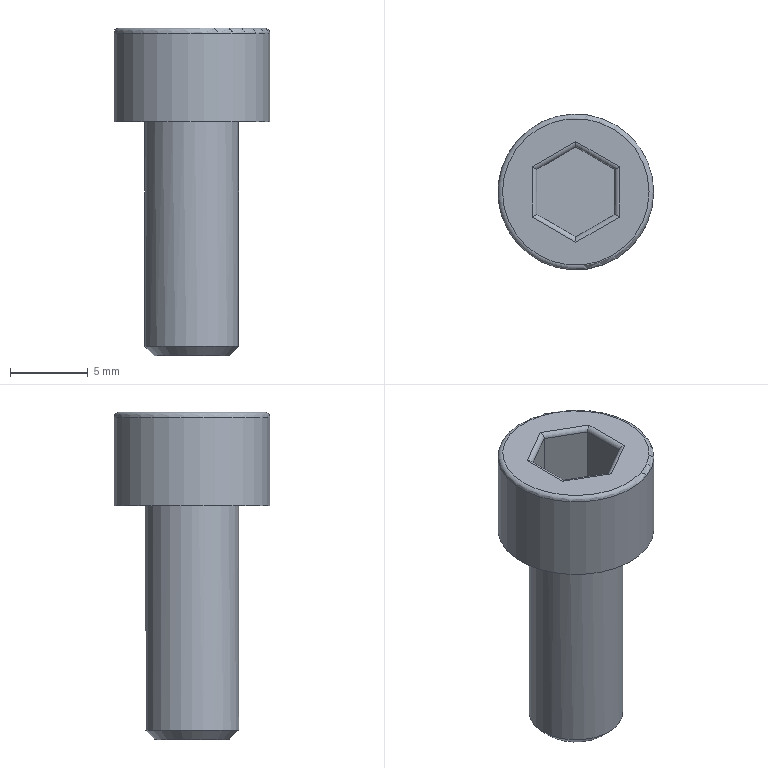Part | STEP file | 200 mesh_id698_x | 1 solid | 20 faces | box 10 x 10 x 21 mm | volume 806.082 mm3 | plane 10 | cylinder 8 | torus 1 | cone 1 | commonest cylinder face diameters 0.6 x6 6.01 x1 10 x1
STEP:
#1=CARTESIAN_POINT('',(-16822.884,-3924.502,11.));
#2=VERTEX_POINT('',#1);
#3=CARTESIAN_POINT('',(-16825.684,-3922.886,11.));
#4=VERTEX_POINT('',#3);
#5=CARTESIAN_POINT('',(-16825.534,-3922.972,11.));
#6=DIRECTION('',(-0.866,0.5,0.));
#7=VECTOR('',#6,1.);
#8=LINE('',#5,#7);
#9=EDGE_CURVE('',#2,#4,#8,.T.);
#10=ORIENTED_EDGE('',*,*,#9,.T.);
#11=CARTESIAN_POINT('',(-16825.684,-3919.653,11.));
#12=VERTEX_POINT('',#11);
#13=CARTESIAN_POINT('',(-16825.684,-3919.826,11.));
#14=DIRECTION('',(0.,1.,0.));
#15=VECTOR('',#14,1.);
#16=LINE('',#13,#15);
#17=EDGE_CURVE('',#4,#12,#16,.T.);
#18=ORIENTED_EDGE('',*,*,#17,.T.);
#19=CARTESIAN_POINT('',(-16822.884,-3918.036,11.));
#20=VERTEX_POINT('',#19);
#21=CARTESIAN_POINT('',(-16823.034,-3918.123,11.));
#22=DIRECTION('',(0.866,0.5,0.));
#23=VECTOR('',#22,1.);
#24=LINE('',#21,#23);
#25=EDGE_CURVE('',#12,#20,#24,.T.);
#26=ORIENTED_EDGE('',*,*,#25,.T.);
#27=CARTESIAN_POINT('',(-16820.084,-3919.653,11.));
#28=VERTEX_POINT('',#27);
#29=CARTESIAN_POINT('',(-16820.234,-3919.566,11.));
#30=DIRECTION('',(0.866,-0.5,0.));
#31=VECTOR('',#30,1.);
#32=LINE('',#29,#31);
#33=EDGE_CURVE('',#20,#28,#32,.T.);
#34=ORIENTED_EDGE('',*,*,#33,.T.);
#35=CARTESIAN_POINT('',(-16820.084,-3922.886,11.));
#36=VERTEX_POINT('',#35);
#37=CARTESIAN_POINT('',(-16820.084,-3922.713,11.));
#38=DIRECTION('',(0.,-1.,0.));
#39=VECTOR('',#38,1.);
#40=LINE('',#37,#39);
#41=EDGE_CURVE('',#28,#36,#40,.T.);
#42=ORIENTED_EDGE('',*,*,#41,.T.);
#43=CARTESIAN_POINT('',(-16822.734,-3924.416,11.));
#44=DIRECTION('',(-0.866,-0.5,0.));
#45=VECTOR('',#44,1.);
#46=LINE('',#43,#45);
#47=EDGE_CURVE('',#36,#2,#46,.T.);
#48=ORIENTED_EDGE('',*,*,#47,.T.);
#49=EDGE_LOOP('',(#10,#18,#26,#34,#42,#48));
#50=FACE_BOUND('',#49,.T.);
#51=CARTESIAN_POINT('',(-16818.184,-3921.269,11.));
#52=VERTEX_POINT('',#51);
#53=CARTESIAN_POINT('',(-16822.884,-3921.269,11.));
#54=DIRECTION('',(0.,0.,1.));
#55=DIRECTION('',(1.,0.,0.));
#56=AXIS2_PLACEMENT_3D('',#53,#54,#55);
#57=CIRCLE('',#56,4.7);
#58=EDGE_CURVE('',#52,#52,#57,.T.);
#59=ORIENTED_EDGE('',*,*,#58,.T.);
#60=EDGE_LOOP('',(#59));
#61=FACE_BOUND('',#60,.T.);
#62=CARTESIAN_POINT('',(-16822.884,-3921.269,11.));
#63=DIRECTION('',(0.,0.,1.));
#64=DIRECTION('',(1.,0.,0.));
#65=AXIS2_PLACEMENT_3D('',#62,#63,#64);
#66=PLANE('',#65);
#67=ADVANCED_FACE('',(#50,#61),#66,.T.);
#68=CARTESIAN_POINT('',(-16825.628,-3922.506,5.));
#69=VERTEX_POINT('',#68);
#70=CARTESIAN_POINT('',(-16825.261,-3923.115,5.));
#71=VERTEX_POINT('',#70);
#72=CARTESIAN_POINT('',(-16822.889,-3921.271,5.));
#73=DIRECTION('',(0.,0.,-1.));
#74=DIRECTION('',(-1.,0.,0.));
#75=AXIS2_PLACEMENT_3D('',#72,#73,#74);
#76=CIRCLE('',#75,3.005);
#77=EDGE_CURVE('',#69,#71,#76,.T.);
#78=ORIENTED_EDGE('',*,*,#77,.F.);
#79=CARTESIAN_POINT('',(-16825.261,-3923.115,5.));
#80=CARTESIAN_POINT('',(-16825.407,-3922.928,5.));
#81=CARTESIAN_POINT('',(-16825.531,-3922.723,5.));
#82=CARTESIAN_POINT('',(-16825.628,-3922.506,5.));
#83=B_SPLINE_CURVE_WITH_KNOTS('',3,(#79,#80,#81,#82),.UNSPECIFIED.,.F.,.F.,(4,4),(0.,1.),.UNSPECIFIED.);
#84=EDGE_CURVE('',#71,#69,#83,.T.);
#85=ORIENTED_EDGE('',*,*,#84,.F.);
#86=EDGE_LOOP('',(#78,#85));
#87=FACE_BOUND('',#86,.T.);
#88=CARTESIAN_POINT('',(-16817.884,-3921.269,5.));
#89=VERTEX_POINT('',#88);
#90=CARTESIAN_POINT('',(-16822.884,-3921.269,5.));
#91=DIRECTION('',(0.,0.,1.));
#92=DIRECTION('',(1.,0.,0.));
#93=AXIS2_PLACEMENT_3D('',#90,#91,#92);
#94=CIRCLE('',#93,5.);
#95=EDGE_CURVE('',#89,#89,#94,.T.);
#96=ORIENTED_EDGE('',*,*,#95,.F.);
#97=EDGE_LOOP('',(#96));
#98=FACE_BOUND('',#97,.T.);
#99=CARTESIAN_POINT('',(-16822.884,-3921.269,5.));
#100=DIRECTION('',(0.,0.,-1.));
#101=DIRECTION('',(-1.,0.,0.));
#102=AXIS2_PLACEMENT_3D('',#99,#100,#101);
#103=PLANE('',#102);
#104=ADVANCED_FACE('',(#87,#98),#103,.T.);
#105=CARTESIAN_POINT('',(-16817.884,-3921.269,10.7));
#106=VERTEX_POINT('',#105);
#107=CARTESIAN_POINT('',(-16822.884,-3921.269,10.7));
#108=DIRECTION('',(0.,0.,-1.));
#109=DIRECTION('',(1.,0.,0.));
#110=AXIS2_PLACEMENT_3D('',#107,#108,#109);
#111=CIRCLE('',#110,5.);
#112=EDGE_CURVE('',#106,#106,#111,.T.);
#113=ORIENTED_EDGE('',*,*,#112,.T.);
#114=EDGE_LOOP('',(#113));
#115=FACE_BOUND('',#114,.T.);
#116=ORIENTED_EDGE('',*,*,#95,.T.);
#117=EDGE_LOOP('',(#116));
#118=FACE_BOUND('',#117,.T.);
#119=CARTESIAN_POINT('',(-16822.884,-3921.269,5.));
#120=DIRECTION('',(0.,0.,1.));
#121=DIRECTION('',(1.,0.,0.));
#122=AXIS2_PLACEMENT_3D('',#119,#120,#121);
#123=CYLINDRICAL_SURFACE('',#122,5.);
#124=ADVANCED_FACE('',(#115,#118),#123,.T.);
#125=ORIENTED_EDGE('',*,*,#58,.F.);
#126=EDGE_LOOP('',(#125));
#127=FACE_BOUND('',#126,.T.);
#128=ORIENTED_EDGE('',*,*,#112,.F.);
#129=EDGE_LOOP('',(#128));
#130=FACE_BOUND('',#129,.T.);
#131=CARTESIAN_POINT('',(-16822.884,-3921.269,10.7));
#132=DIRECTION('',(0.,0.,1.));
#133=DIRECTION('',(1.,0.,0.));
#134=AXIS2_PLACEMENT_3D('',#131,#132,#133);
#135=TOROIDAL_SURFACE('',#134,4.7,0.3);
#136=ADVANCED_FACE('',(#127,#130),#135,.T.);
#137=CARTESIAN_POINT('',(-16822.884,-3924.156,10.7));
#138=VERTEX_POINT('',#137);
#139=CARTESIAN_POINT('',(-16822.884,-3924.156,7.));
#140=VERTEX_POINT('',#139);
#141=CARTESIAN_POINT('',(-16822.884,-3924.156,7.));
#142=DIRECTION('',(0.,0.,-1.));
#143=VECTOR('',#142,1.);
#144=LINE('',#141,#143);
#145=EDGE_CURVE('',#138,#140,#144,.T.);
#146=ORIENTED_EDGE('',*,*,#145,.F.);
#147=CARTESIAN_POINT('',(-16820.384,-3922.713,10.7));
#148=VERTEX_POINT('',#147);
#149=CARTESIAN_POINT('',(-16820.384,-3922.713,10.7));
#150=DIRECTION('',(0.866,0.5,0.));
#151=VECTOR('',#150,1.);
#152=LINE('',#149,#151);
#153=EDGE_CURVE('',#138,#148,#152,.T.);
#154=ORIENTED_EDGE('',*,*,#153,.T.);
#155=CARTESIAN_POINT('',(-16820.384,-3922.713,7.));
#156=VERTEX_POINT('',#155);
#157=CARTESIAN_POINT('',(-16820.384,-3922.713,7.));
#158=DIRECTION('',(0.,0.,-1.));
#159=VECTOR('',#158,1.);
#160=LINE('',#157,#159);
#161=EDGE_CURVE('',#148,#156,#160,.T.);
#162=ORIENTED_EDGE('',*,*,#161,.T.);
#163=CARTESIAN_POINT('',(-16822.884,-3924.156,7.));
#164=DIRECTION('',(-0.866,-0.5,0.));
#165=VECTOR('',#164,1.);
#166=LINE('',#163,#165);
#167=EDGE_CURVE('',#156,#140,#166,.T.);
#168=ORIENTED_EDGE('',*,*,#167,.T.);
#169=EDGE_LOOP('',(#146,#154,#162,#168));
#170=FACE_OUTER_BOUND('',#169,.T.);
#171=CARTESIAN_POINT('',(-16822.884,-3924.156,7.));
#172=DIRECTION('',(0.5,-0.866,0.));
#173=DIRECTION('',(0.866,0.5,0.));
#174=AXIS2_PLACEMENT_3D('',#171,#172,#173);
#175=PLANE('',#174);
#176=ADVANCED_FACE('',(#170),#175,.F.);
#177=ORIENTED_EDGE('',*,*,#161,.F.);
#178=CARTESIAN_POINT('',(-16820.384,-3919.826,10.7));
#179=VERTEX_POINT('',#178);
#180=CARTESIAN_POINT('',(-16820.384,-3919.826,10.7));
#181=DIRECTION('',(0.,1.,0.));
#182=VECTOR('',#181,1.);
#183=LINE('',#180,#182);
#184=EDGE_CURVE('',#148,#179,#183,.T.);
#185=ORIENTED_EDGE('',*,*,#184,.T.);
#186=CARTESIAN_POINT('',(-16820.384,-3919.826,7.));
#187=VERTEX_POINT('',#186);
#188=CARTESIAN_POINT('',(-16820.384,-3919.826,7.));
#189=DIRECTION('',(0.,0.,-1.));
#190=VECTOR('',#189,1.);
#191=LINE('',#188,#190);
#192=EDGE_CURVE('',#179,#187,#191,.T.);
#193=ORIENTED_EDGE('',*,*,#192,.T.);
#194=CARTESIAN_POINT('',(-16820.384,-3922.713,7.));
#195=DIRECTION('',(0.,-1.,0.));
#196=VECTOR('',#195,1.);
#197=LINE('',#194,#196);
#198=EDGE_CURVE('',#187,#156,#197,.T.);
#199=ORIENTED_EDGE('',*,*,#198,.T.);
#200=EDGE_LOOP('',(#177,#185,#193,#199));
#201=FACE_OUTER_BOUND('',#200,.T.);
#202=CARTESIAN_POINT('',(-16820.384,-3922.713,7.));
#203=DIRECTION('',(1.,0.,0.));
#204=DIRECTION('',(0.,0.,-1.));
#205=AXIS2_PLACEMENT_3D('',#202,#203,#204);
#206=PLANE('',#205);
#207=ADVANCED_FACE('',(#201),#206,.F.);
#208=ORIENTED_EDGE('',*,*,#192,.F.);
#209=CARTESIAN_POINT('',(-16822.884,-3918.382,10.7));
#210=VERTEX_POINT('',#209);
#211=CARTESIAN_POINT('',(-16822.884,-3918.382,10.7));
#212=DIRECTION('',(-0.866,0.5,0.));
#213=VECTOR('',#212,1.);
#214=LINE('',#211,#213);
#215=EDGE_CURVE('',#179,#210,#214,.T.);
#216=ORIENTED_EDGE('',*,*,#215,.T.);
#217=CARTESIAN_POINT('',(-16822.884,-3918.382,7.));
#218=VERTEX_POINT('',#217);
#219=CARTESIAN_POINT('',(-16822.884,-3918.382,7.));
#220=DIRECTION('',(0.,0.,-1.));
#221=VECTOR('',#220,1.);
#222=LINE('',#219,#221);
#223=EDGE_CURVE('',#210,#218,#222,.T.);
#224=ORIENTED_EDGE('',*,*,#223,.T.);
#225=CARTESIAN_POINT('',(-16820.384,-3919.826,7.));
#226=DIRECTION('',(0.866,-0.5,0.));
#227=VECTOR('',#226,1.);
#228=LINE('',#225,#227);
#229=EDGE_CURVE('',#218,#187,#228,.T.);
#230=ORIENTED_EDGE('',*,*,#229,.T.);
#231=EDGE_LOOP('',(#208,#216,#224,#230));
#232=FACE_OUTER_BOUND('',#231,.T.);
#233=CARTESIAN_POINT('',(-16820.384,-3919.826,7.));
#234=DIRECTION('',(0.5,0.866,0.));
#235=DIRECTION('',(-0.866,0.5,0.));
#236=AXIS2_PLACEMENT_3D('',#233,#234,#235);
#237=PLANE('',#236);
#238=ADVANCED_FACE('',(#232),#237,.F.);
#239=ORIENTED_EDGE('',*,*,#223,.F.);
#240=CARTESIAN_POINT('',(-16825.384,-3919.826,10.7));
#241=VERTEX_POINT('',#240);
#242=CARTESIAN_POINT('',(-16825.384,-3919.826,10.7));
#243=DIRECTION('',(-0.866,-0.5,0.));
#244=VECTOR('',#243,1.);
#245=LINE('',#242,#244);
#246=EDGE_CURVE('',#210,#241,#245,.T.);
#247=ORIENTED_EDGE('',*,*,#246,.T.);
#248=CARTESIAN_POINT('',(-16825.384,-3919.826,7.));
#249=VERTEX_POINT('',#248);
#250=CARTESIAN_POINT('',(-16825.384,-3919.826,7.));
#251=DIRECTION('',(0.,0.,-1.));
#252=VECTOR('',#251,1.);
#253=LINE('',#250,#252);
#254=EDGE_CURVE('',#241,#249,#253,.T.);
#255=ORIENTED_EDGE('',*,*,#254,.T.);
#256=CARTESIAN_POINT('',(-16822.884,-3918.382,7.));
#257=DIRECTION('',(0.866,0.5,0.));
#258=VECTOR('',#257,1.);
#259=LINE('',#256,#258);
#260=EDGE_CURVE('',#249,#218,#259,.T.);
#261=ORIENTED_EDGE('',*,*,#260,.T.);
#262=EDGE_LOOP('',(#239,#247,#255,#261));
#263=FACE_OUTER_BOUND('',#262,.T.);
#264=CARTESIAN_POINT('',(-16822.884,-3918.382,7.));
#265=DIRECTION('',(-0.5,0.866,0.));
#266=DIRECTION('',(-0.866,-0.5,0.));
#267=AXIS2_PLACEMENT_3D('',#264,#265,#266);
#268=PLANE('',#267);
#269=ADVANCED_FACE('',(#263),#268,.F.);
#270=ORIENTED_EDGE('',*,*,#254,.F.);
#271=CARTESIAN_POINT('',(-16825.384,-3922.713,10.7));
#272=VERTEX_POINT('',#271);
#273=CARTESIAN_POINT('',(-16825.384,-3922.713,10.7));
#274=DIRECTION('',(0.,-1.,0.));
#275=VECTOR('',#274,1.);
#276=LINE('',#273,#275);
#277=EDGE_CURVE('',#241,#272,#276,.T.);
#278=ORIENTED_EDGE('',*,*,#277,.T.);
#279=CARTESIAN_POINT('',(-16825.384,-3922.713,7.));
#280=VERTEX_POINT('',#279);
#281=CARTESIAN_POINT('',(-16825.384,-3922.713,7.));
#282=DIRECTION('',(0.,0.,-1.));
#283=VECTOR('',#282,1.);
#284=LINE('',#281,#283);
#285=EDGE_CURVE('',#272,#280,#284,.T.);
#286=ORIENTED_EDGE('',*,*,#285,.T.);
#287=CARTESIAN_POINT('',(-16825.384,-3919.826,7.));
#288=DIRECTION('',(0.,1.,0.));
#289=VECTOR('',#288,1.);
#290=LINE('',#287,#289);
#291=EDGE_CURVE('',#280,#249,#290,.T.);
#292=ORIENTED_EDGE('',*,*,#291,.T.);
#293=EDGE_LOOP('',(#270,#278,#286,#292));
#294=FACE_OUTER_BOUND('',#293,.T.);
#295=CARTESIAN_POINT('',(-16825.384,-3919.826,7.));
#296=DIRECTION('',(-1.,0.,0.));
#297=DIRECTION('',(0.,0.,1.));
#298=AXIS2_PLACEMENT_3D('',#295,#296,#297);
#299=PLANE('',#298);
#300=ADVANCED_FACE('',(#294),#299,.F.);
#301=ORIENTED_EDGE('',*,*,#285,.F.);
#302=CARTESIAN_POINT('',(-16822.884,-3924.156,10.7));
#303=DIRECTION('',(0.866,-0.5,0.));
#304=VECTOR('',#303,1.);
#305=LINE('',#302,#304);
#306=EDGE_CURVE('',#272,#138,#305,.T.);
#307=ORIENTED_EDGE('',*,*,#306,.T.);
#308=ORIENTED_EDGE('',*,*,#145,.T.);
#309=CARTESIAN_POINT('',(-16825.384,-3922.713,7.));
#310=DIRECTION('',(-0.866,0.5,0.));
#311=VECTOR('',#310,1.);
#312=LINE('',#309,#311);
#313=EDGE_CURVE('',#140,#280,#312,.T.);
#314=ORIENTED_EDGE('',*,*,#313,.T.);
#315=EDGE_LOOP('',(#301,#307,#308,#314));
#316=FACE_OUTER_BOUND('',#315,.T.);
#317=CARTESIAN_POINT('',(-16825.384,-3922.713,7.));
#318=DIRECTION('',(-0.5,-0.866,0.));
#319=DIRECTION('',(0.866,-0.5,0.));
#320=AXIS2_PLACEMENT_3D('',#317,#318,#319);
#321=PLANE('',#320);
#322=ADVANCED_FACE('',(#316),#321,.F.);
#323=ORIENTED_EDGE('',*,*,#167,.F.);
#324=ORIENTED_EDGE('',*,*,#198,.F.);
#325=ORIENTED_EDGE('',*,*,#229,.F.);
#326=ORIENTED_EDGE('',*,*,#260,.F.);
#327=ORIENTED_EDGE('',*,*,#291,.F.);
#328=ORIENTED_EDGE('',*,*,#313,.F.);
#329=EDGE_LOOP('',(#323,#324,#325,#326,#327,#328));
#330=FACE_OUTER_BOUND('',#329,.T.);
#331=CARTESIAN_POINT('',(181.514,26.,7.));
#332=DIRECTION('',(0.,0.,1.));
#333=DIRECTION('',(1.,0.,0.));
#334=AXIS2_PLACEMENT_3D('',#331,#332,#333);
#335=PLANE('',#334);
#336=ADVANCED_FACE('',(#330),#335,.T.);
#337=CARTESIAN_POINT('',(-16820.084,-3922.886,10.7));
#338=DIRECTION('',(-0.5,-0.866,0.));
#339=DIRECTION('',(-0.866,0.5,0.));
#340=AXIS2_PLACEMENT_3D('',#337,#338,#339);
#341=ELLIPSE('',#340,0.3464,0.3);
#342=EDGE_CURVE('',#36,#148,#341,.T.);
#343=ORIENTED_EDGE('',*,*,#342,.F.);
#344=ORIENTED_EDGE('',*,*,#41,.F.);
#345=CARTESIAN_POINT('',(-16820.084,-3919.653,10.7));
#346=DIRECTION('',(-0.5,0.866,0.));
#347=DIRECTION('',(-0.866,-0.5,0.));
#348=AXIS2_PLACEMENT_3D('',#345,#346,#347);
#349=ELLIPSE('',#348,0.3464,0.3);
#350=EDGE_CURVE('',#179,#28,#349,.T.);
#351=ORIENTED_EDGE('',*,*,#350,.F.);
#352=ORIENTED_EDGE('',*,*,#184,.F.);
#353=EDGE_LOOP('',(#343,#344,#351,#352));
#354=FACE_OUTER_BOUND('',#353,.T.);
#355=CARTESIAN_POINT('',(-16820.084,-3922.713,10.7));
#356=DIRECTION('',(0.,-1.,0.));
#357=DIRECTION('',(0.,0.,-1.));
#358=AXIS2_PLACEMENT_3D('',#355,#356,#357);
#359=CYLINDRICAL_SURFACE('',#358,0.3);
#360=ADVANCED_FACE('',(#354),#359,.T.);
#361=ORIENTED_EDGE('',*,*,#350,.T.);
#362=ORIENTED_EDGE('',*,*,#33,.F.);
#363=CARTESIAN_POINT('',(-16822.884,-3918.036,10.7));
#364=DIRECTION('',(-1.,0.,0.));
#365=DIRECTION('',(0.,1.,0.));
#366=AXIS2_PLACEMENT_3D('',#363,#364,#365);
#367=ELLIPSE('',#366,0.3464,0.3);
#368=EDGE_CURVE('',#210,#20,#367,.T.);
#369=ORIENTED_EDGE('',*,*,#368,.F.);
#370=ORIENTED_EDGE('',*,*,#215,.F.);
#371=EDGE_LOOP('',(#361,#362,#369,#370));
#372=FACE_OUTER_BOUND('',#371,.T.);
#373=CARTESIAN_POINT('',(-16820.234,-3919.566,10.7));
#374=DIRECTION('',(0.866,-0.5,0.));
#375=DIRECTION('',(0.5,0.866,0.));
#376=AXIS2_PLACEMENT_3D('',#373,#374,#375);
#377=CYLINDRICAL_SURFACE('',#376,0.3);
#378=ADVANCED_FACE('',(#372),#377,.T.);
#379=ORIENTED_EDGE('',*,*,#342,.T.);
#380=ORIENTED_EDGE('',*,*,#153,.F.);
#381=CARTESIAN_POINT('',(-16822.884,-3924.502,10.7));
#382=DIRECTION('',(-1.,0.,0.));
#383=DIRECTION('',(0.,1.,0.));
#384=AXIS2_PLACEMENT_3D('',#381,#382,#383);
#385=ELLIPSE('',#384,0.3464,0.3);
#386=EDGE_CURVE('',#2,#138,#385,.T.);
#387=ORIENTED_EDGE('',*,*,#386,.F.);
#388=ORIENTED_EDGE('',*,*,#47,.F.);
#389=EDGE_LOOP('',(#379,#380,#387,#388));
#390=FACE_OUTER_BOUND('',#389,.T.);
#391=CARTESIAN_POINT('',(-16822.734,-3924.416,10.7));
#392=DIRECTION('',(-0.866,-0.5,0.));
#393=DIRECTION('',(0.5,-0.866,0.));
#394=AXIS2_PLACEMENT_3D('',#391,#392,#393);
#395=CYLINDRICAL_SURFACE('',#394,0.3);
#396=ADVANCED_FACE('',(#390),#395,.T.);
#397=ORIENTED_EDGE('',*,*,#368,.T.);
#398=ORIENTED_EDGE('',*,*,#25,.F.);
#399=CARTESIAN_POINT('',(-16825.684,-3919.653,10.7));
#400=DIRECTION('',(-0.5,-0.866,0.));
#401=DIRECTION('',(-0.866,0.5,0.));
#402=AXIS2_PLACEMENT_3D('',#399,#400,#401);
#403=ELLIPSE('',#402,0.3464,0.3);
#404=EDGE_CURVE('',#241,#12,#403,.T.);
#405=ORIENTED_EDGE('',*,*,#404,.F.);
#406=ORIENTED_EDGE('',*,*,#246,.F.);
#407=EDGE_LOOP('',(#397,#398,#405,#406));
#408=FACE_OUTER_BOUND('',#407,.T.);
#409=CARTESIAN_POINT('',(-16823.034,-3918.123,10.7));
#410=DIRECTION('',(0.866,0.5,0.));
#411=DIRECTION('',(-0.5,0.866,0.));
#412=AXIS2_PLACEMENT_3D('',#409,#410,#411);
#413=CYLINDRICAL_SURFACE('',#412,0.3);
#414=ADVANCED_FACE('',(#408),#413,.T.);
#415=ORIENTED_EDGE('',*,*,#386,.T.);
#416=ORIENTED_EDGE('',*,*,#306,.F.);
#417=CARTESIAN_POINT('',(-16825.684,-3922.886,10.7));
#418=DIRECTION('',(-0.5,0.866,0.));
#419=DIRECTION('',(0.866,0.5,0.));
#420=AXIS2_PLACEMENT_3D('',#417,#418,#419);
#421=ELLIPSE('',#420,0.3464,0.3);
#422=EDGE_CURVE('',#4,#272,#421,.T.);
#423=ORIENTED_EDGE('',*,*,#422,.F.);
#424=ORIENTED_EDGE('',*,*,#9,.F.);
#425=EDGE_LOOP('',(#415,#416,#423,#424));
#426=FACE_OUTER_BOUND('',#425,.T.);
#427=CARTESIAN_POINT('',(-16825.534,-3922.972,10.7));
#428=DIRECTION('',(-0.866,0.5,0.));
#429=DIRECTION('',(-0.5,-0.866,0.));
#430=AXIS2_PLACEMENT_3D('',#427,#428,#429);
#431=CYLINDRICAL_SURFACE('',#430,0.3);
#432=ADVANCED_FACE('',(#426),#431,.T.);
#433=ORIENTED_EDGE('',*,*,#404,.T.);
#434=ORIENTED_EDGE('',*,*,#17,.F.);
#435=ORIENTED_EDGE('',*,*,#422,.T.);
#436=ORIENTED_EDGE('',*,*,#277,.F.);
#437=EDGE_LOOP('',(#433,#434,#435,#436));
#438=FACE_OUTER_BOUND('',#437,.T.);
#439=CARTESIAN_POINT('',(-16825.684,-3919.826,10.7));
#440=DIRECTION('',(0.,1.,0.));
#441=DIRECTION('',(0.,0.,1.));
#442=AXIS2_PLACEMENT_3D('',#439,#440,#441);
#443=CYLINDRICAL_SURFACE('',#442,0.3);
#444=ADVANCED_FACE('',(#438),#443,.T.);
#445=CARTESIAN_POINT('',(-16825.894,-3921.271,-9.4));
#446=VERTEX_POINT('',#445);
#447=CARTESIAN_POINT('',(-16822.889,-3921.271,-9.4));
#448=DIRECTION('',(0.,0.,1.));
#449=DIRECTION('',(-1.,0.,0.));
#450=AXIS2_PLACEMENT_3D('',#447,#448,#449);
#451=CIRCLE('',#450,3.005);
#452=EDGE_CURVE('',#446,#446,#451,.T.);
#453=ORIENTED_EDGE('',*,*,#452,.T.);
#454=EDGE_LOOP('',(#453));
#455=FACE_BOUND('',#454,.T.);
#456=ORIENTED_EDGE('',*,*,#77,.T.);
#457=ORIENTED_EDGE('',*,*,#84,.T.);
#458=EDGE_LOOP('',(#456,#457));
#459=FACE_BOUND('',#458,.T.);
#460=CARTESIAN_POINT('',(-16822.889,-3921.271,-10.));
#461=DIRECTION('',(0.,0.,1.));
#462=DIRECTION('',(0.866,0.5,0.));
#463=AXIS2_PLACEMENT_3D('',#460,#461,#462);
#464=CYLINDRICAL_SURFACE('',#463,3.005);
#465=ADVANCED_FACE('',(#455,#459),#464,.T.);
#466=CARTESIAN_POINT('',(-16825.294,-3921.271,-10.));
#467=VERTEX_POINT('',#466);
#468=CARTESIAN_POINT('',(-16822.889,-3921.271,-10.));
#469=DIRECTION('',(0.,0.,-1.));
#470=DIRECTION('',(-1.,0.,0.));
#471=AXIS2_PLACEMENT_3D('',#468,#469,#470);
#472=CIRCLE('',#471,2.405);
#473=EDGE_CURVE('',#467,#467,#472,.T.);
#474=ORIENTED_EDGE('',*,*,#473,.T.);
#475=EDGE_LOOP('',(#474));
#476=FACE_OUTER_BOUND('',#475,.T.);
#477=CARTESIAN_POINT('',(-16822.884,-3921.269,-10.));
#478=DIRECTION('',(0.,0.,-1.));
#479=DIRECTION('',(-1.,0.,0.));
#480=AXIS2_PLACEMENT_3D('',#477,#478,#479);
#481=PLANE('',#480);
#482=ADVANCED_FACE('',(#476),#481,.T.);
#483=ORIENTED_EDGE('',*,*,#473,.F.);
#484=EDGE_LOOP('',(#483));
#485=FACE_BOUND('',#484,.T.);
#486=ORIENTED_EDGE('',*,*,#452,.F.);
#487=EDGE_LOOP('',(#486));
#488=FACE_BOUND('',#487,.T.);
#489=CARTESIAN_POINT('',(-16822.889,-3921.271,-9.4));
#490=DIRECTION('',(0.,0.,1.));
#491=DIRECTION('',(1.,0.,0.));
#492=AXIS2_PLACEMENT_3D('',#489,#490,#491);
#493=CONICAL_SURFACE('',#492,3.005,45.);
#494=ADVANCED_FACE('',(#485,#488),#493,.T.);
#495=CLOSED_SHELL('',(#67,#104,#124,#136,#176,#207,#238,#269,#300,#322,#336,#360,#378,#396,#414,#432,#444,#465,#482,#494));
#496=MANIFOLD_SOLID_BREP('',#495);
#497=(LENGTH_UNIT()NAMED_UNIT(*)SI_UNIT(.MILLI.,.METRE.));
#498=UNCERTAINTY_MEASURE_WITH_UNIT(LENGTH_MEASURE(0.0508),#497,'','');
#499=(NAMED_UNIT(*)PLANE_ANGLE_UNIT()SI_UNIT($,.RADIAN.));
#500=PLANE_ANGLE_MEASURE_WITH_UNIT(PLANE_ANGLE_MEASURE(0.01745),#499);
#501=DIMENSIONAL_EXPONENTS(0.,0.,0.,0.,0.,0.,0.);
#502=(CONVERSION_BASED_UNIT('DEGREE',#500)NAMED_UNIT(#501)PLANE_ANGLE_UNIT());
#503=(NAMED_UNIT(*)SI_UNIT($,.STERADIAN.)SOLID_ANGLE_UNIT());
#504=(GEOMETRIC_REPRESENTATION_CONTEXT(3)GLOBAL_UNCERTAINTY_ASSIGNED_CONTEXT((#498))GLOBAL_UNIT_ASSIGNED_CONTEXT((#497,#502,#503))REPRESENTATION_CONTEXT('',''));
#505=ADVANCED_BREP_SHAPE_REPRESENTATION('',(#496),#504);